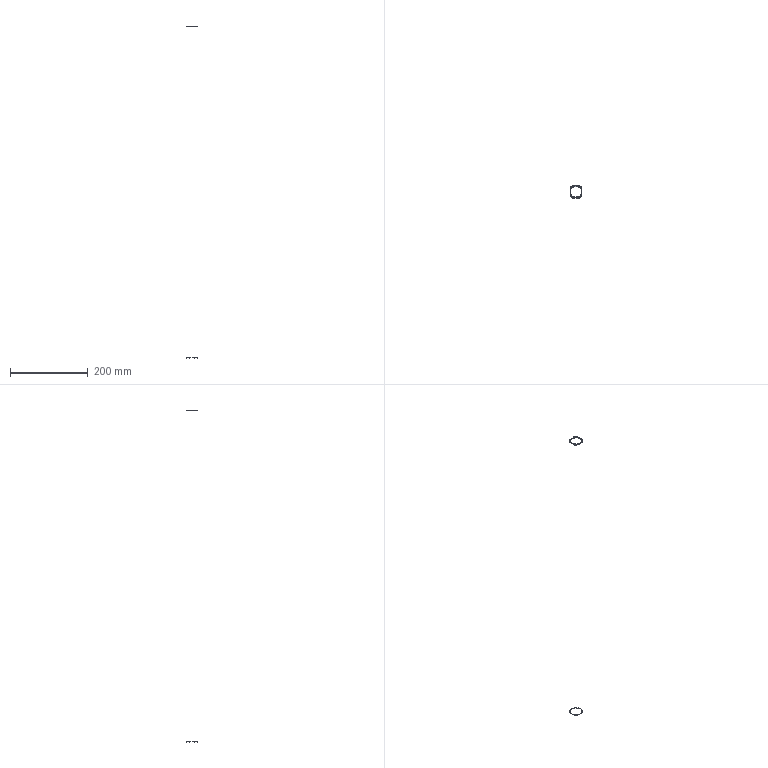Part | SolidWorks | features BaseBody 5 | 5 solids | 57 faces | box 30 x 30 x 855 mm | volume 277.779 mm3 | cylinder 22 | plane 21 | cone 14 | commonest cylinder face diameters 15 x14 9 x8